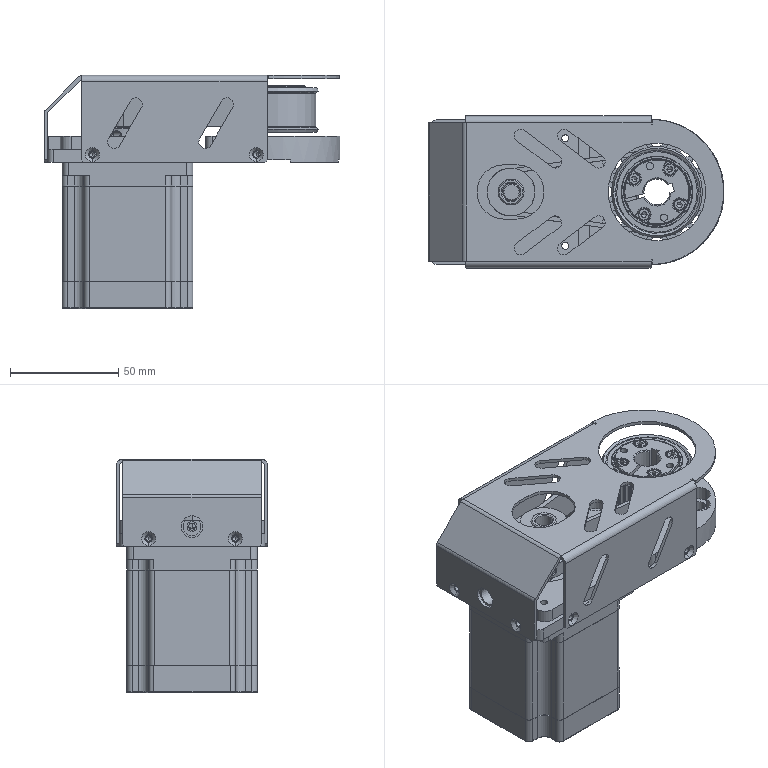Part | STEP file | Copy of C0045-60 side link 2:1(K60)^K50A-1H20-S(formula driven)-L300-motor left- | 13 solids | 1010 faces | box 136.5 x 70 x 107.5 mm | volume 331047 mm3 | cylinder 584 | plane 265 | cone 125 | spline 32 | torus 4 | commonest cylinder face diameters 0.6 x161 1.82 x90 37.44 x40 6 x38 5 x24 19.1 x21